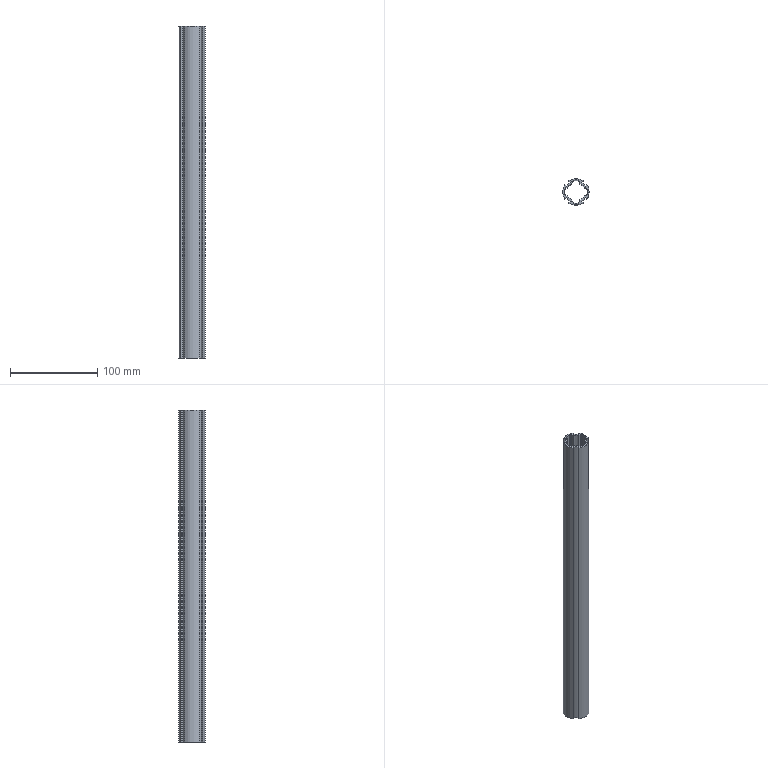Part | STEP file | DROP STOP 1 ALUMINUM_Default<As machined> | 1 solid | 52 faces | box 30 x 30 x 380 mm | volume 75887 mm3 | cylinder 26 | plane 26 | commonest cylinder face diameters 24.6 x8 27 x5 30 x5 21 x4 25 x4